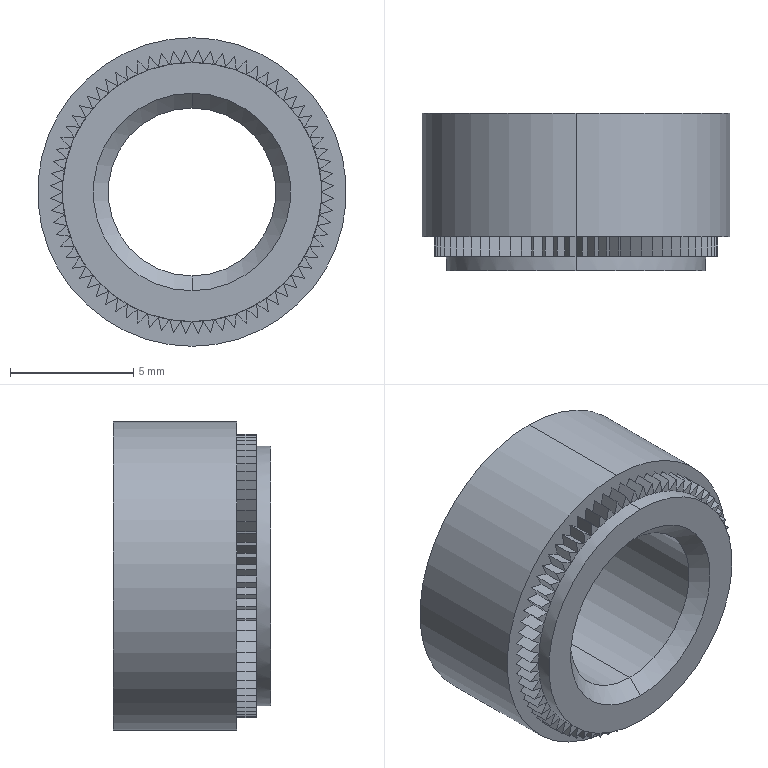Part | STEP file | 921292560 | 1 solid | 229 faces | box 12.5 x 6.38 x 12.5 mm | volume 499.816 mm3 | plane 219 | cylinder 6 | cone 4 | commonest cylinder face diameters 6.8 x2 10.5 x2 12.5 x2